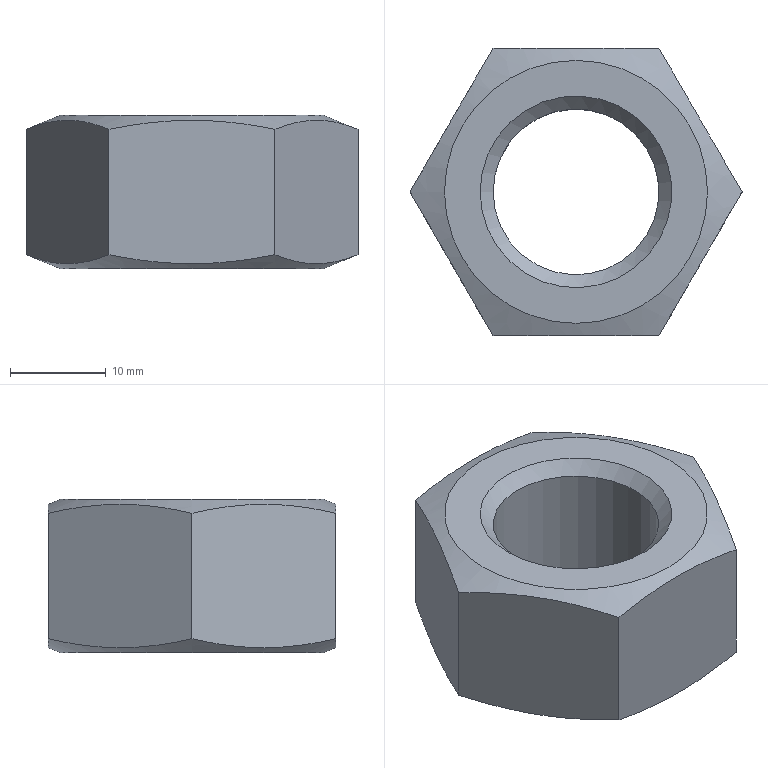Part | STEP file | 1_28 | 1 solid | 13 faces | box 34.641 x 30 x 16 mm | volume 8431 mm3 | plane 8 | cone 4 | cylinder 1 | commonest cylinder face diameters 17.294 x1
STEP:
#1=CARTESIAN_POINT('',(0.,0.,0.));
#2=DIRECTION('',(0.,0.,1.));
#3=DIRECTION('',(1.,0.,0.));
#4=AXIS2_PLACEMENT_3D('',#1,#2,#3);
#5=CARTESIAN_POINT('',(-8.647,0.,1.353));
#6=VERTEX_POINT('',#5);
#7=CARTESIAN_POINT('',(0.,0.,1.353));
#8=DIRECTION('',(0.,0.,-1.));
#9=DIRECTION('',(1.,0.,0.));
#10=AXIS2_PLACEMENT_3D('',#7,#8,#9);
#11=CIRCLE('',#10,8.647);
#12=CARTESIAN_POINT('',(0.,0.,0.6766));
#13=DIRECTION('',(0.,0.,-1.));
#14=DIRECTION('',(1.,0.,0.));
#15=AXIS2_PLACEMENT_3D('',#12,#13,#14);
#16=CONICAL_SURFACE('',#15,9.323,0.7854);
#17=CARTESIAN_POINT('',(0.,-0.6766));
#18=DIRECTION('',(1.,0.));
#19=VECTOR('',#18,1.);
#20=LINE('',#17,#19);
#21=(GEOMETRIC_REPRESENTATION_CONTEXT(2)PARAMETRIC_REPRESENTATION_CONTEXT()REPRESENTATION_CONTEXT('',''));
#22=DEFINITIONAL_REPRESENTATION('',(#20),#21);
#23=PCURVE('',#16,#22);
#24=CARTESIAN_POINT('',(0.,0.,8.));
#25=DIRECTION('',(0.,0.,-1.));
#26=DIRECTION('',(1.,0.,0.));
#27=AXIS2_PLACEMENT_3D('',#24,#25,#26);
#28=CYLINDRICAL_SURFACE('',#27,8.647);
#29=CARTESIAN_POINT('',(0.,6.647));
#30=DIRECTION('',(1.,0.));
#31=VECTOR('',#30,1.);
#32=LINE('',#29,#31);
#33=(GEOMETRIC_REPRESENTATION_CONTEXT(2)PARAMETRIC_REPRESENTATION_CONTEXT()REPRESENTATION_CONTEXT('',''));
#34=DEFINITIONAL_REPRESENTATION('',(#32),#33);
#35=PCURVE('',#28,#34);
#36=SURFACE_CURVE('',#11,(#23,#35),.PCURVE_S1.);
#37=EDGE_CURVE('',#6,#6,#36,.T.);
#38=ORIENTED_EDGE('',*,*,#37,.T.);
#39=CARTESIAN_POINT('',(-10.,0.,0.));
#40=VERTEX_POINT('',#39);
#41=CARTESIAN_POINT('',(-8.647,0.,1.353));
#42=CARTESIAN_POINT('',(-10.,0.,-0.000000001));
#43=B_SPLINE_CURVE_WITH_KNOTS('',1,(#41,#42),.UNSPECIFIED.,.F.,.F.,(2,2),(-0.9568,0.9568),.PIECEWISE_BEZIER_KNOTS.);
#44=CARTESIAN_POINT('',(9.425,0.));
#45=DIRECTION('',(0.,1.));
#46=VECTOR('',#45,1.);
#47=LINE('',#44,#46);
#48=(GEOMETRIC_REPRESENTATION_CONTEXT(2)PARAMETRIC_REPRESENTATION_CONTEXT()REPRESENTATION_CONTEXT('',''));
#49=DEFINITIONAL_REPRESENTATION('',(#47),#48);
#50=PCURVE('',#16,#49);
#51=CARTESIAN_POINT('',(3.142,0.));
#52=DIRECTION('',(0.,1.));
#53=VECTOR('',#52,1.);
#54=LINE('',#51,#53);
#55=(GEOMETRIC_REPRESENTATION_CONTEXT(2)PARAMETRIC_REPRESENTATION_CONTEXT()REPRESENTATION_CONTEXT('',''));
#56=DEFINITIONAL_REPRESENTATION('',(#54),#55);
#57=PCURVE('',#16,#56);
#58=SEAM_CURVE('',#43,(#50,#57),.PCURVE_S1.);
#59=EDGE_CURVE('',#6,#40,#58,.T.);
#60=ORIENTED_EDGE('',*,*,#59,.T.);
#61=CARTESIAN_POINT('',(0.,0.,0.));
#62=DIRECTION('',(0.,0.,-1.));
#63=DIRECTION('',(1.,0.,0.));
#64=AXIS2_PLACEMENT_3D('',#61,#62,#63);
#65=CIRCLE('',#64,10.);
#66=CARTESIAN_POINT('',(0.,0.6766));
#67=DIRECTION('',(1.,0.));
#68=VECTOR('',#67,1.);
#69=LINE('',#66,#68);
#70=(GEOMETRIC_REPRESENTATION_CONTEXT(2)PARAMETRIC_REPRESENTATION_CONTEXT()REPRESENTATION_CONTEXT('',''));
#71=DEFINITIONAL_REPRESENTATION('',(#69),#70);
#72=PCURVE('',#16,#71);
#73=CARTESIAN_POINT('',(0.,0.,0.));
#74=DIRECTION('',(0.,0.,1.));
#75=DIRECTION('',(1.,0.,0.));
#76=AXIS2_PLACEMENT_3D('',#73,#74,#75);
#77=PLANE('',#76);
#78=CARTESIAN_POINT('',(10.,0.));
#79=CARTESIAN_POINT('',(10.,-17.321));
#80=CARTESIAN_POINT('',(-5.,-8.66));
#81=CARTESIAN_POINT('',(-20.,0.));
#82=CARTESIAN_POINT('',(-5.,8.66));
#83=CARTESIAN_POINT('',(10.,17.321));
#84=CARTESIAN_POINT('',(10.,0.));
#85=(BOUNDED_CURVE()B_SPLINE_CURVE(2,(#78,#79,#80,#81,#82,#83,#84),.UNSPECIFIED.,.T.,.F.)B_SPLINE_CURVE_WITH_KNOTS((1,2,2,2,2,1),(-2.094,0.,2.094,4.189,6.283,8.378),.UNSPECIFIED.)CURVE()GEOMETRIC_REPRESENTATION_ITEM()RATIONAL_B_SPLINE_CURVE((1.,0.5,1.,0.5,1.,0.5,1.))REPRESENTATION_ITEM(''));
#86=(GEOMETRIC_REPRESENTATION_CONTEXT(2)PARAMETRIC_REPRESENTATION_CONTEXT()REPRESENTATION_CONTEXT('',''));
#87=DEFINITIONAL_REPRESENTATION('',(#85),#86);
#88=PCURVE('',#77,#87);
#89=SURFACE_CURVE('',#65,(#72,#88),.PCURVE_S1.);
#90=EDGE_CURVE('',#40,#40,#89,.T.);
#91=ORIENTED_EDGE('',*,*,#90,.F.);
#92=ORIENTED_EDGE('',*,*,#59,.F.);
#93=EDGE_LOOP('',(#38,#60,#91,#92));
#94=FACE_BOUND('',#93,.F.);
#95=ADVANCED_FACE('',(#94),#16,.F.);
#96=CARTESIAN_POINT('',(-13.72,0.,0.));
#97=VERTEX_POINT('',#96);
#98=CARTESIAN_POINT('',(0.,0.,0.));
#99=DIRECTION('',(0.,0.,1.));
#100=DIRECTION('',(1.,0.,0.));
#101=AXIS2_PLACEMENT_3D('',#98,#99,#100);
#102=CIRCLE('',#101,13.72);
#103=CARTESIAN_POINT('',(0.,0.));
#104=DIRECTION('',(1.,0.));
#105=AXIS2_PLACEMENT_2D('',#103,#104);
#106=CIRCLE('',#105,13.72);
#107=(GEOMETRIC_REPRESENTATION_CONTEXT(2)PARAMETRIC_REPRESENTATION_CONTEXT()REPRESENTATION_CONTEXT('',''));
#108=DEFINITIONAL_REPRESENTATION('',(#106),#107);
#109=PCURVE('',#77,#108);
#110=CARTESIAN_POINT('',(0.,0.,0.7273));
#111=DIRECTION('',(0.,0.,1.));
#112=DIRECTION('',(1.,0.,0.));
#113=AXIS2_PLACEMENT_3D('',#110,#111,#112);
#114=CONICAL_SURFACE('',#113,15.52,1.187);
#115=CARTESIAN_POINT('',(0.,-0.7273));
#116=DIRECTION('',(1.,0.));
#117=VECTOR('',#116,1.);
#118=LINE('',#115,#117);
#119=(GEOMETRIC_REPRESENTATION_CONTEXT(2)PARAMETRIC_REPRESENTATION_CONTEXT()REPRESENTATION_CONTEXT('',''));
#120=DEFINITIONAL_REPRESENTATION('',(#118),#119);
#121=PCURVE('',#114,#120);
#122=SURFACE_CURVE('',#102,(#109,#121),.PCURVE_S1.);
#123=EDGE_CURVE('',#97,#97,#122,.T.);
#124=ORIENTED_EDGE('',*,*,#123,.F.);
#125=EDGE_LOOP('',(#124));
#126=FACE_BOUND('',#125,.T.);
#127=ORIENTED_EDGE('',*,*,#90,.F.);
#128=EDGE_LOOP('',(#127));
#129=FACE_BOUND('',#128,.T.);
#130=ADVANCED_FACE('',(#126,#129),#77,.F.);
#131=CARTESIAN_POINT('',(-8.647,0.,14.647));
#132=VERTEX_POINT('',#131);
#133=CARTESIAN_POINT('',(0.,0.,14.647));
#134=DIRECTION('',(0.,0.,-1.));
#135=DIRECTION('',(1.,0.,0.));
#136=AXIS2_PLACEMENT_3D('',#133,#134,#135);
#137=CIRCLE('',#136,8.647);
#138=CARTESIAN_POINT('',(0.,-6.647));
#139=DIRECTION('',(1.,0.));
#140=VECTOR('',#139,1.);
#141=LINE('',#138,#140);
#142=(GEOMETRIC_REPRESENTATION_CONTEXT(2)PARAMETRIC_REPRESENTATION_CONTEXT()REPRESENTATION_CONTEXT('',''));
#143=DEFINITIONAL_REPRESENTATION('',(#141),#142);
#144=PCURVE('',#28,#143);
#145=CARTESIAN_POINT('',(0.,0.,15.323));
#146=DIRECTION('',(0.,0.,1.));
#147=DIRECTION('',(-1.,0.,0.));
#148=AXIS2_PLACEMENT_3D('',#145,#146,#147);
#149=CONICAL_SURFACE('',#148,9.323,0.7854);
#150=CARTESIAN_POINT('',(9.425,-0.6766));
#151=DIRECTION('',(-1.,0.));
#152=VECTOR('',#151,1.);
#153=LINE('',#150,#152);
#154=(GEOMETRIC_REPRESENTATION_CONTEXT(2)PARAMETRIC_REPRESENTATION_CONTEXT()REPRESENTATION_CONTEXT('',''));
#155=DEFINITIONAL_REPRESENTATION('',(#153),#154);
#156=PCURVE('',#149,#155);
#157=SURFACE_CURVE('',#137,(#144,#156),.PCURVE_S1.);
#158=EDGE_CURVE('',#132,#132,#157,.T.);
#159=ORIENTED_EDGE('',*,*,#158,.T.);
#160=CARTESIAN_POINT('',(-8.647,0.,14.647));
#161=CARTESIAN_POINT('',(-8.647,0.,1.353));
#162=B_SPLINE_CURVE_WITH_KNOTS('',1,(#160,#161),.UNSPECIFIED.,.F.,.F.,(2,2),(-6.647,6.647),.PIECEWISE_BEZIER_KNOTS.);
#163=CARTESIAN_POINT('',(9.425,0.));
#164=DIRECTION('',(0.,1.));
#165=VECTOR('',#164,1.);
#166=LINE('',#163,#165);
#167=(GEOMETRIC_REPRESENTATION_CONTEXT(2)PARAMETRIC_REPRESENTATION_CONTEXT()REPRESENTATION_CONTEXT('',''));
#168=DEFINITIONAL_REPRESENTATION('',(#166),#167);
#169=PCURVE('',#28,#168);
#170=CARTESIAN_POINT('',(3.142,0.));
#171=DIRECTION('',(0.,1.));
#172=VECTOR('',#171,1.);
#173=LINE('',#170,#172);
#174=(GEOMETRIC_REPRESENTATION_CONTEXT(2)PARAMETRIC_REPRESENTATION_CONTEXT()REPRESENTATION_CONTEXT('',''));
#175=DEFINITIONAL_REPRESENTATION('',(#173),#174);
#176=PCURVE('',#28,#175);
#177=SEAM_CURVE('',#162,(#169,#176),.PCURVE_S1.);
#178=EDGE_CURVE('',#132,#6,#177,.T.);
#179=ORIENTED_EDGE('',*,*,#178,.T.);
#180=ORIENTED_EDGE('',*,*,#37,.F.);
#181=ORIENTED_EDGE('',*,*,#178,.F.);
#182=EDGE_LOOP('',(#159,#179,#180,#181));
#183=FACE_BOUND('',#182,.F.);
#184=ADVANCED_FACE('',(#183),#28,.F.);
#185=CARTESIAN_POINT('',(-17.32,0.,1.455));
#186=VERTEX_POINT('',#185);
#187=CARTESIAN_POINT('',(-8.66,15.,1.455));
#188=VERTEX_POINT('',#187);
#189=CARTESIAN_POINT('',(-39.287,-38.047,16.553));
#190=CARTESIAN_POINT('',(-12.99,7.5,-3.881));
#191=CARTESIAN_POINT('',(13.306,53.047,16.553));
#192=(BOUNDED_CURVE()B_SPLINE_CURVE(2,(#189,#190,#191),.UNSPECIFIED.,.F.,.F.)B_SPLINE_CURVE_WITH_KNOTS((3,3),(0.,10.997),.PIECEWISE_BEZIER_KNOTS.)CURVE()GEOMETRIC_REPRESENTATION_ITEM()RATIONAL_B_SPLINE_CURVE((1.,3.646,1.))REPRESENTATION_ITEM(''));
#193=CARTESIAN_POINT('',(9.425,0.7273));
#194=CARTESIAN_POINT('',(9.41,0.6661));
#195=CARTESIAN_POINT('',(9.379,0.5509));
#196=CARTESIAN_POINT('',(9.333,0.3985));
#197=CARTESIAN_POINT('',(9.286,0.2652));
#198=CARTESIAN_POINT('',(9.239,0.1498));
#199=CARTESIAN_POINT('',(9.191,0.05157));
#200=CARTESIAN_POINT('',(9.144,-0.03038));
#201=CARTESIAN_POINT('',(9.095,-0.09663));
#202=CARTESIAN_POINT('',(9.047,-0.1477));
#203=CARTESIAN_POINT('',(8.999,-0.1839));
#204=CARTESIAN_POINT('',(8.95,-0.2055));
#205=CARTESIAN_POINT('',(8.901,-0.2127));
#206=CARTESIAN_POINT('',(8.852,-0.2055));
#207=CARTESIAN_POINT('',(8.804,-0.1839));
#208=CARTESIAN_POINT('',(8.755,-0.1477));
#209=CARTESIAN_POINT('',(8.707,-0.09663));
#210=CARTESIAN_POINT('',(8.659,-0.03038));
#211=CARTESIAN_POINT('',(8.611,0.05157));
#212=CARTESIAN_POINT('',(8.563,0.1498));
#213=CARTESIAN_POINT('',(8.516,0.2652));
#214=CARTESIAN_POINT('',(8.469,0.3985));
#215=CARTESIAN_POINT('',(8.423,0.5509));
#216=CARTESIAN_POINT('',(8.393,0.6661));
#217=CARTESIAN_POINT('',(8.378,0.7273));
#218=B_SPLINE_CURVE_WITH_KNOTS('',3,(#193,#194,#195,#196,#197,#198,#199,#200,#201,#202,#203,#204,#205,#206,#207,#208,#209,#210,#211,#212,#213,#214,#215,#216,#217),.UNSPECIFIED.,.F.,.F.,(4,1,1,1,1,1,1,1,1,1,1,1,1,1,1,1,1,1,1,1,1,1,4),(3.546,3.724,3.901,4.079,4.256,4.434,4.611,4.788,4.966,5.143,5.321,5.498,5.676,5.853,6.031,6.208,6.386,6.563,6.741,6.918,7.096,7.273,7.451),.QUASI_UNIFORM_KNOTS.);
#219=(GEOMETRIC_REPRESENTATION_CONTEXT(2)PARAMETRIC_REPRESENTATION_CONTEXT()REPRESENTATION_CONTEXT('',''));
#220=DEFINITIONAL_REPRESENTATION('',(#218),#219);
#221=PCURVE('',#114,#220);
#222=CARTESIAN_POINT('',(-17.32,0.,0.));
#223=DIRECTION('',(-0.866,0.5,0.));
#224=DIRECTION('',(0.,0.,1.));
#225=AXIS2_PLACEMENT_3D('',#222,#223,#224);
#226=PLANE('',#225);
#227=CARTESIAN_POINT('',(16.553,-43.933));
#228=CARTESIAN_POINT('',(-3.881,8.66));
#229=CARTESIAN_POINT('',(16.553,61.253));
#230=(BOUNDED_CURVE()B_SPLINE_CURVE(2,(#227,#228,#229),.UNSPECIFIED.,.F.,.F.)B_SPLINE_CURVE_WITH_KNOTS((3,3),(0.,10.997),.PIECEWISE_BEZIER_KNOTS.)CURVE()GEOMETRIC_REPRESENTATION_ITEM()RATIONAL_B_SPLINE_CURVE((1.,3.646,1.))REPRESENTATION_ITEM(''));
#231=(GEOMETRIC_REPRESENTATION_CONTEXT(2)PARAMETRIC_REPRESENTATION_CONTEXT()REPRESENTATION_CONTEXT('',''));
#232=DEFINITIONAL_REPRESENTATION('',(#230),#231);
#233=PCURVE('',#226,#232);
#234=SURFACE_CURVE('',#192,(#221,#233),.PCURVE_S1.);
#235=EDGE_CURVE('',#186,#188,#234,.T.);
#236=ORIENTED_EDGE('',*,*,#235,.T.);
#237=CARTESIAN_POINT('',(8.66,15.,1.455));
#238=VERTEX_POINT('',#237);
#239=CARTESIAN_POINT('',(-52.593,15.,16.553));
#240=CARTESIAN_POINT('',(0.,15.,-3.881));
#241=CARTESIAN_POINT('',(52.593,15.,16.553));
#242=(BOUNDED_CURVE()B_SPLINE_CURVE(2,(#239,#240,#241),.UNSPECIFIED.,.F.,.F.)B_SPLINE_CURVE_WITH_KNOTS((3,3),(0.,10.997),.PIECEWISE_BEZIER_KNOTS.)CURVE()GEOMETRIC_REPRESENTATION_ITEM()RATIONAL_B_SPLINE_CURVE((1.,3.646,1.))REPRESENTATION_ITEM(''));
#243=CARTESIAN_POINT('',(8.378,0.7273));
#244=CARTESIAN_POINT('',(8.362,0.6661));
#245=CARTESIAN_POINT('',(8.332,0.5509));
#246=CARTESIAN_POINT('',(8.286,0.3985));
#247=CARTESIAN_POINT('',(8.239,0.2652));
#248=CARTESIAN_POINT('',(8.192,0.1498));
#249=CARTESIAN_POINT('',(8.144,0.05157));
#250=CARTESIAN_POINT('',(8.096,-0.03038));
#251=CARTESIAN_POINT('',(8.048,-0.09663));
#252=CARTESIAN_POINT('',(8.,-0.1477));
#253=CARTESIAN_POINT('',(7.951,-0.1839));
#254=CARTESIAN_POINT('',(7.903,-0.2055));
#255=CARTESIAN_POINT('',(7.854,-0.2127));
#256=CARTESIAN_POINT('',(7.805,-0.2055));
#257=CARTESIAN_POINT('',(7.757,-0.1839));
#258=CARTESIAN_POINT('',(7.708,-0.1477));
#259=CARTESIAN_POINT('',(7.66,-0.09663));
#260=CARTESIAN_POINT('',(7.612,-0.03038));
#261=CARTESIAN_POINT('',(7.564,0.05157));
#262=CARTESIAN_POINT('',(7.516,0.1498));
#263=CARTESIAN_POINT('',(7.469,0.2652));
#264=CARTESIAN_POINT('',(7.422,0.3985));
#265=CARTESIAN_POINT('',(7.376,0.5509));
#266=CARTESIAN_POINT('',(7.346,0.6661));
#267=CARTESIAN_POINT('',(7.33,0.7273));
#268=B_SPLINE_CURVE_WITH_KNOTS('',3,(#243,#244,#245,#246,#247,#248,#249,#250,#251,#252,#253,#254,#255,#256,#257,#258,#259,#260,#261,#262,#263,#264,#265,#266,#267),.UNSPECIFIED.,.F.,.F.,(4,1,1,1,1,1,1,1,1,1,1,1,1,1,1,1,1,1,1,1,1,1,4),(3.546,3.724,3.901,4.079,4.256,4.434,4.611,4.788,4.966,5.143,5.321,5.498,5.676,5.853,6.031,6.208,6.386,6.563,6.741,6.918,7.096,7.273,7.451),.QUASI_UNIFORM_KNOTS.);
#269=(GEOMETRIC_REPRESENTATION_CONTEXT(2)PARAMETRIC_REPRESENTATION_CONTEXT()REPRESENTATION_CONTEXT('',''));
#270=DEFINITIONAL_REPRESENTATION('',(#268),#269);
#271=PCURVE('',#114,#270);
#272=CARTESIAN_POINT('',(-8.66,15.,0.));
#273=DIRECTION('',(0.,1.,0.));
#274=DIRECTION('',(0.,0.,1.));
#275=AXIS2_PLACEMENT_3D('',#272,#273,#274);
#276=PLANE('',#275);
#277=CARTESIAN_POINT('',(16.553,-43.933));
#278=CARTESIAN_POINT('',(-3.881,8.66));
#279=CARTESIAN_POINT('',(16.553,61.253));
#280=(BOUNDED_CURVE()B_SPLINE_CURVE(2,(#277,#278,#279),.UNSPECIFIED.,.F.,.F.)B_SPLINE_CURVE_WITH_KNOTS((3,3),(0.,10.997),.PIECEWISE_BEZIER_KNOTS.)CURVE()GEOMETRIC_REPRESENTATION_ITEM()RATIONAL_B_SPLINE_CURVE((1.,3.646,1.))REPRESENTATION_ITEM(''));
#281=(GEOMETRIC_REPRESENTATION_CONTEXT(2)PARAMETRIC_REPRESENTATION_CONTEXT()REPRESENTATION_CONTEXT('',''));
#282=DEFINITIONAL_REPRESENTATION('',(#280),#281);
#283=PCURVE('',#276,#282);
#284=SURFACE_CURVE('',#242,(#271,#283),.PCURVE_S1.);
#285=EDGE_CURVE('',#188,#238,#284,.T.);
#286=ORIENTED_EDGE('',*,*,#285,.T.);
#287=CARTESIAN_POINT('',(17.32,0.,1.455));
#288=VERTEX_POINT('',#287);
#289=CARTESIAN_POINT('',(-13.306,53.047,16.553));
#290=CARTESIAN_POINT('',(12.99,7.5,-3.881));
#291=CARTESIAN_POINT('',(39.287,-38.047,16.553));
#292=(BOUNDED_CURVE()B_SPLINE_CURVE(2,(#289,#290,#291),.UNSPECIFIED.,.F.,.F.)B_SPLINE_CURVE_WITH_KNOTS((3,3),(0.,10.997),.PIECEWISE_BEZIER_KNOTS.)CURVE()GEOMETRIC_REPRESENTATION_ITEM()RATIONAL_B_SPLINE_CURVE((1.,3.646,1.))REPRESENTATION_ITEM(''));
#293=CARTESIAN_POINT('',(7.33,0.7273));
#294=CARTESIAN_POINT('',(7.315,0.6661));
#295=CARTESIAN_POINT('',(7.285,0.5509));
#296=CARTESIAN_POINT('',(7.238,0.3985));
#297=CARTESIAN_POINT('',(7.192,0.2652));
#298=CARTESIAN_POINT('',(7.145,0.1498));
#299=CARTESIAN_POINT('',(7.097,0.05157));
#300=CARTESIAN_POINT('',(7.049,-0.03038));
#301=CARTESIAN_POINT('',(7.001,-0.09663));
#302=CARTESIAN_POINT('',(6.953,-0.1477));
#303=CARTESIAN_POINT('',(6.904,-0.1839));
#304=CARTESIAN_POINT('',(6.856,-0.2055));
#305=CARTESIAN_POINT('',(6.807,-0.2127));
#306=CARTESIAN_POINT('',(6.758,-0.2055));
#307=CARTESIAN_POINT('',(6.709,-0.1839));
#308=CARTESIAN_POINT('',(6.661,-0.1477));
#309=CARTESIAN_POINT('',(6.612,-0.09663));
#310=CARTESIAN_POINT('',(6.564,-0.03038));
#311=CARTESIAN_POINT('',(6.516,0.05157));
#312=CARTESIAN_POINT('',(6.469,0.1498));
#313=CARTESIAN_POINT('',(6.422,0.2652));
#314=CARTESIAN_POINT('',(6.375,0.3985));
#315=CARTESIAN_POINT('',(6.329,0.5509));
#316=CARTESIAN_POINT('',(6.298,0.6661));
#317=CARTESIAN_POINT('',(6.283,0.7273));
#318=B_SPLINE_CURVE_WITH_KNOTS('',3,(#293,#294,#295,#296,#297,#298,#299,#300,#301,#302,#303,#304,#305,#306,#307,#308,#309,#310,#311,#312,#313,#314,#315,#316,#317),.UNSPECIFIED.,.F.,.F.,(4,1,1,1,1,1,1,1,1,1,1,1,1,1,1,1,1,1,1,1,1,1,4),(3.546,3.724,3.901,4.079,4.256,4.434,4.611,4.788,4.966,5.143,5.321,5.498,5.676,5.853,6.031,6.208,6.386,6.563,6.741,6.918,7.096,7.273,7.451),.QUASI_UNIFORM_KNOTS.);
#319=(GEOMETRIC_REPRESENTATION_CONTEXT(2)PARAMETRIC_REPRESENTATION_CONTEXT()REPRESENTATION_CONTEXT('',''));
#320=DEFINITIONAL_REPRESENTATION('',(#318),#319);
#321=PCURVE('',#114,#320);
#322=CARTESIAN_POINT('',(8.66,15.,0.));
#323=DIRECTION('',(0.866,0.5,0.));
#324=DIRECTION('',(0.,0.,-1.));
#325=AXIS2_PLACEMENT_3D('',#322,#323,#324);
#326=PLANE('',#325);
#327=CARTESIAN_POINT('',(-16.553,43.933));
#328=CARTESIAN_POINT('',(3.881,-8.66));
#329=CARTESIAN_POINT('',(-16.553,-61.253));
#330=(BOUNDED_CURVE()B_SPLINE_CURVE(2,(#327,#328,#329),.UNSPECIFIED.,.F.,.F.)B_SPLINE_CURVE_WITH_KNOTS((3,3),(0.,10.997),.PIECEWISE_BEZIER_KNOTS.)CURVE()GEOMETRIC_REPRESENTATION_ITEM()RATIONAL_B_SPLINE_CURVE((1.,3.646,1.))REPRESENTATION_ITEM(''));
#331=(GEOMETRIC_REPRESENTATION_CONTEXT(2)PARAMETRIC_REPRESENTATION_CONTEXT()REPRESENTATION_CONTEXT('',''));
#332=DEFINITIONAL_REPRESENTATION('',(#330),#331);
#333=PCURVE('',#326,#332);
#334=SURFACE_CURVE('',#292,(#321,#333),.PCURVE_S1.);
#335=EDGE_CURVE('',#238,#288,#334,.T.);
#336=ORIENTED_EDGE('',*,*,#335,.T.);
#337=CARTESIAN_POINT('',(8.66,-15.,1.455));
#338=VERTEX_POINT('',#337);
#339=CARTESIAN_POINT('',(39.287,38.047,16.553));
#340=CARTESIAN_POINT('',(12.99,-7.5,-3.881));
#341=CARTESIAN_POINT('',(-13.306,-53.047,16.553));
#342=(BOUNDED_CURVE()B_SPLINE_CURVE(2,(#339,#340,#341),.UNSPECIFIED.,.F.,.F.)B_SPLINE_CURVE_WITH_KNOTS((3,3),(0.,10.997),.PIECEWISE_BEZIER_KNOTS.)CURVE()GEOMETRIC_REPRESENTATION_ITEM()RATIONAL_B_SPLINE_CURVE((1.,3.646,1.))REPRESENTATION_ITEM(''));
#343=CARTESIAN_POINT('',(6.283,0.7273));
#344=CARTESIAN_POINT('',(6.268,0.6661));
#345=CARTESIAN_POINT('',(6.238,0.5509));
#346=CARTESIAN_POINT('',(6.191,0.3985));
#347=CARTESIAN_POINT('',(6.145,0.2652));
#348=CARTESIAN_POINT('',(6.097,0.1498));
#349=CARTESIAN_POINT('',(6.05,0.05157));
#350=CARTESIAN_POINT('',(6.002,-0.03038));
#351=CARTESIAN_POINT('',(5.954,-0.09663));
#352=CARTESIAN_POINT('',(5.906,-0.1477));
#353=CARTESIAN_POINT('',(5.857,-0.1839));
#354=CARTESIAN_POINT('',(5.808,-0.2055));
#355=CARTESIAN_POINT('',(5.76,-0.2127));
#356=CARTESIAN_POINT('',(5.711,-0.2055));
#357=CARTESIAN_POINT('',(5.662,-0.1839));
#358=CARTESIAN_POINT('',(5.614,-0.1477));
#359=CARTESIAN_POINT('',(5.565,-0.09663));
#360=CARTESIAN_POINT('',(5.517,-0.03038));
#361=CARTESIAN_POINT('',(5.469,0.05157));
#362=CARTESIAN_POINT('',(5.422,0.1498));
#363=CARTESIAN_POINT('',(5.375,0.2652));
#364=CARTESIAN_POINT('',(5.328,0.3985));
#365=CARTESIAN_POINT('',(5.282,0.5509));
#366=CARTESIAN_POINT('',(5.251,0.6661));
#367=CARTESIAN_POINT('',(5.236,0.7273));
#368=B_SPLINE_CURVE_WITH_KNOTS('',3,(#343,#344,#345,#346,#347,#348,#349,#350,#351,#352,#353,#354,#355,#356,#357,#358,#359,#360,#361,#362,#363,#364,#365,#366,#367),.UNSPECIFIED.,.F.,.F.,(4,1,1,1,1,1,1,1,1,1,1,1,1,1,1,1,1,1,1,1,1,1,4),(3.546,3.724,3.901,4.079,4.256,4.434,4.611,4.788,4.966,5.143,5.321,5.498,5.676,5.853,6.031,6.208,6.386,6.563,6.741,6.918,7.096,7.273,7.451),.QUASI_UNIFORM_KNOTS.);
#369=(GEOMETRIC_REPRESENTATION_CONTEXT(2)PARAMETRIC_REPRESENTATION_CONTEXT()REPRESENTATION_CONTEXT('',''));
#370=DEFINITIONAL_REPRESENTATION('',(#368),#369);
#371=PCURVE('',#114,#370);
#372=CARTESIAN_POINT('',(17.32,0.,0.));
#373=DIRECTION('',(0.866,-0.5,0.));
#374=DIRECTION('',(0.,0.,-1.));
#375=AXIS2_PLACEMENT_3D('',#372,#373,#374);
#376=PLANE('',#375);
#377=CARTESIAN_POINT('',(-16.553,43.933));
#378=CARTESIAN_POINT('',(3.881,-8.66));
#379=CARTESIAN_POINT('',(-16.553,-61.253));
#380=(BOUNDED_CURVE()B_SPLINE_CURVE(2,(#377,#378,#379),.UNSPECIFIED.,.F.,.F.)B_SPLINE_CURVE_WITH_KNOTS((3,3),(0.,10.997),.PIECEWISE_BEZIER_KNOTS.)CURVE()GEOMETRIC_REPRESENTATION_ITEM()RATIONAL_B_SPLINE_CURVE((1.,3.646,1.))REPRESENTATION_ITEM(''));
#381=(GEOMETRIC_REPRESENTATION_CONTEXT(2)PARAMETRIC_REPRESENTATION_CONTEXT()REPRESENTATION_CONTEXT('',''));
#382=DEFINITIONAL_REPRESENTATION('',(#380),#381);
#383=PCURVE('',#376,#382);
#384=SURFACE_CURVE('',#342,(#371,#383),.PCURVE_S1.);
#385=EDGE_CURVE('',#288,#338,#384,.T.);
#386=ORIENTED_EDGE('',*,*,#385,.T.);
#387=CARTESIAN_POINT('',(-8.66,-15.,1.455));
#388=VERTEX_POINT('',#387);
#389=CARTESIAN_POINT('',(52.593,-15.,16.553));
#390=CARTESIAN_POINT('',(0.,-15.,-3.881));
#391=CARTESIAN_POINT('',(-52.593,-15.,16.553));
#392=(BOUNDED_CURVE()B_SPLINE_CURVE(2,(#389,#390,#391),.UNSPECIFIED.,.F.,.F.)B_SPLINE_CURVE_WITH_KNOTS((3,3),(0.,10.997),.PIECEWISE_BEZIER_KNOTS.)CURVE()GEOMETRIC_REPRESENTATION_ITEM()RATIONAL_B_SPLINE_CURVE((1.,3.646,1.))REPRESENTATION_ITEM(''));
#393=CARTESIAN_POINT('',(5.236,0.7273));
#394=CARTESIAN_POINT('',(5.221,0.6661));
#395=CARTESIAN_POINT('',(5.19,0.5509));
#396=CARTESIAN_POINT('',(5.144,0.3985));
#397=CARTESIAN_POINT('',(5.097,0.2652));
#398=CARTESIAN_POINT('',(5.05,0.1498));
#399=CARTESIAN_POINT('',(5.003,0.05157));
#400=CARTESIAN_POINT('',(4.955,-0.03038));
#401=CARTESIAN_POINT('',(4.907,-0.09663));
#402=CARTESIAN_POINT('',(4.858,-0.1477));
#403=CARTESIAN_POINT('',(4.81,-0.1839));
#404=CARTESIAN_POINT('',(4.761,-0.2055));
#405=CARTESIAN_POINT('',(4.712,-0.2127));
#406=CARTESIAN_POINT('',(4.664,-0.2055));
#407=CARTESIAN_POINT('',(4.615,-0.1839));
#408=CARTESIAN_POINT('',(4.566,-0.1477));
#409=CARTESIAN_POINT('',(4.518,-0.09663));
#410=CARTESIAN_POINT('',(4.47,-0.03038));
#411=CARTESIAN_POINT('',(4.422,0.05157));
#412=CARTESIAN_POINT('',(4.375,0.1498));
#413=CARTESIAN_POINT('',(4.327,0.2652));
#414=CARTESIAN_POINT('',(4.281,0.3985));
#415=CARTESIAN_POINT('',(4.234,0.5509));
#416=CARTESIAN_POINT('',(4.204,0.6661));
#417=CARTESIAN_POINT('',(4.189,0.7273));
#418=B_SPLINE_CURVE_WITH_KNOTS('',3,(#393,#394,#395,#396,#397,#398,#399,#400,#401,#402,#403,#404,#405,#406,#407,#408,#409,#410,#411,#412,#413,#414,#415,#416,#417),.UNSPECIFIED.,.F.,.F.,(4,1,1,1,1,1,1,1,1,1,1,1,1,1,1,1,1,1,1,1,1,1,4),(3.546,3.724,3.901,4.079,4.256,4.434,4.611,4.788,4.966,5.143,5.321,5.498,5.676,5.853,6.031,6.208,6.386,6.563,6.741,6.918,7.096,7.273,7.451),.QUASI_UNIFORM_KNOTS.);
#419=(GEOMETRIC_REPRESENTATION_CONTEXT(2)PARAMETRIC_REPRESENTATION_CONTEXT()REPRESENTATION_CONTEXT('',''));
#420=DEFINITIONAL_REPRESENTATION('',(#418),#419);
#421=PCURVE('',#114,#420);
#422=CARTESIAN_POINT('',(8.66,-15.,0.));
#423=DIRECTION('',(0.,-1.,0.));
#424=DIRECTION('',(0.,0.,-1.));
#425=AXIS2_PLACEMENT_3D('',#422,#423,#424);
#426=PLANE('',#425);
#427=CARTESIAN_POINT('',(-16.553,43.933));
#428=CARTESIAN_POINT('',(3.881,-8.66));
#429=CARTESIAN_POINT('',(-16.553,-61.253));
#430=(BOUNDED_CURVE()B_SPLINE_CURVE(2,(#427,#428,#429),.UNSPECIFIED.,.F.,.F.)B_SPLINE_CURVE_WITH_KNOTS((3,3),(0.,10.997),.PIECEWISE_BEZIER_KNOTS.)CURVE()GEOMETRIC_REPRESENTATION_ITEM()RATIONAL_B_SPLINE_CURVE((1.,3.646,1.))REPRESENTATION_ITEM(''));
#431=(GEOMETRIC_REPRESENTATION_CONTEXT(2)PARAMETRIC_REPRESENTATION_CONTEXT()REPRESENTATION_CONTEXT('',''));
#432=DEFINITIONAL_REPRESENTATION('',(#430),#431);
#433=PCURVE('',#426,#432);
#434=SURFACE_CURVE('',#392,(#421,#433),.PCURVE_S1.);
#435=EDGE_CURVE('',#338,#388,#434,.T.);
#436=ORIENTED_EDGE('',*,*,#435,.T.);
#437=CARTESIAN_POINT('',(13.306,-53.047,16.553));
#438=CARTESIAN_POINT('',(-12.99,-7.5,-3.881));
#439=CARTESIAN_POINT('',(-39.287,38.047,16.553));
#440=(BOUNDED_CURVE()B_SPLINE_CURVE(2,(#437,#438,#439),.UNSPECIFIED.,.F.,.F.)B_SPLINE_CURVE_WITH_KNOTS((3,3),(0.,10.997),.PIECEWISE_BEZIER_KNOTS.)CURVE()GEOMETRIC_REPRESENTATION_ITEM()RATIONAL_B_SPLINE_CURVE((1.,3.646,1.))REPRESENTATION_ITEM(''));
#441=CARTESIAN_POINT('',(4.189,0.7273));
#442=CARTESIAN_POINT('',(4.174,0.6661));
#443=CARTESIAN_POINT('',(4.143,0.5509));
#444=CARTESIAN_POINT('',(4.097,0.3985));
#445=CARTESIAN_POINT('',(4.05,0.2652));
#446=CARTESIAN_POINT('',(4.003,0.1498));
#447=CARTESIAN_POINT('',(3.956,0.05157));
#448=CARTESIAN_POINT('',(3.908,-0.03038));
#449=CARTESIAN_POINT('',(3.859,-0.09663));
#450=CARTESIAN_POINT('',(3.811,-0.1477));
#451=CARTESIAN_POINT('',(3.763,-0.1839));
#452=CARTESIAN_POINT('',(3.714,-0.2055));
#453=CARTESIAN_POINT('',(3.665,-0.2127));
#454=CARTESIAN_POINT('',(3.616,-0.2055));
#455=CARTESIAN_POINT('',(3.568,-0.1839));
#456=CARTESIAN_POINT('',(3.519,-0.1477));
#457=CARTESIAN_POINT('',(3.471,-0.09663));
#458=CARTESIAN_POINT('',(3.423,-0.03038));
#459=CARTESIAN_POINT('',(3.375,0.05157));
#460=CARTESIAN_POINT('',(3.327,0.1498));
#461=CARTESIAN_POINT('',(3.28,0.2652));
#462=CARTESIAN_POINT('',(3.233,0.3985));
#463=CARTESIAN_POINT('',(3.187,0.5509));
#464=CARTESIAN_POINT('',(3.157,0.6661));
#465=CARTESIAN_POINT('',(3.142,0.7273));
#466=B_SPLINE_CURVE_WITH_KNOTS('',3,(#441,#442,#443,#444,#445,#446,#447,#448,#449,#450,#451,#452,#453,#454,#455,#456,#457,#458,#459,#460,#461,#462,#463,#464,#465),.UNSPECIFIED.,.F.,.F.,(4,1,1,1,1,1,1,1,1,1,1,1,1,1,1,1,1,1,1,1,1,1,4),(3.546,3.724,3.901,4.079,4.256,4.434,4.611,4.788,4.966,5.143,5.321,5.498,5.676,5.853,6.031,6.208,6.386,6.563,6.741,6.918,7.096,7.273,7.451),.QUASI_UNIFORM_KNOTS.);
#467=(GEOMETRIC_REPRESENTATION_CONTEXT(2)PARAMETRIC_REPRESENTATION_CONTEXT()REPRESENTATION_CONTEXT('',''));
#468=DEFINITIONAL_REPRESENTATION('',(#466),#467);
#469=PCURVE('',#114,#468);
#470=CARTESIAN_POINT('',(-8.66,-15.,0.));
#471=DIRECTION('',(-0.866,-0.5,0.));
#472=DIRECTION('',(0.,0.,1.));
#473=AXIS2_PLACEMENT_3D('',#470,#471,#472);
#474=PLANE('',#473);
#475=CARTESIAN_POINT('',(16.553,-43.933));
#476=CARTESIAN_POINT('',(-3.881,8.66));
#477=CARTESIAN_POINT('',(16.553,61.253));
#478=(BOUNDED_CURVE()B_SPLINE_CURVE(2,(#475,#476,#477),.UNSPECIFIED.,.F.,.F.)B_SPLINE_CURVE_WITH_KNOTS((3,3),(0.,10.997),.PIECEWISE_BEZIER_KNOTS.)CURVE()GEOMETRIC_REPRESENTATION_ITEM()RATIONAL_B_SPLINE_CURVE((1.,3.646,1.))REPRESENTATION_ITEM(''));
#479=(GEOMETRIC_REPRESENTATION_CONTEXT(2)PARAMETRIC_REPRESENTATION_CONTEXT()REPRESENTATION_CONTEXT('',''));
#480=DEFINITIONAL_REPRESENTATION('',(#478),#479);
#481=PCURVE('',#474,#480);
#482=SURFACE_CURVE('',#440,(#469,#481),.PCURVE_S1.);
#483=EDGE_CURVE('',#388,#186,#482,.T.);
#484=ORIENTED_EDGE('',*,*,#483,.T.);
#485=CARTESIAN_POINT('',(-13.72,0.,-0.000000002));
#486=CARTESIAN_POINT('',(-17.32,0.,1.455));
#487=B_SPLINE_CURVE_WITH_KNOTS('',1,(#485,#486),.UNSPECIFIED.,.F.,.F.,(2,2),(-1.941,1.941),.PIECEWISE_BEZIER_KNOTS.);
#488=CARTESIAN_POINT('',(3.142,0.));
#489=DIRECTION('',(0.,1.));
#490=VECTOR('',#489,1.);
#491=LINE('',#488,#490);
#492=(GEOMETRIC_REPRESENTATION_CONTEXT(2)PARAMETRIC_REPRESENTATION_CONTEXT()REPRESENTATION_CONTEXT('',''));
#493=DEFINITIONAL_REPRESENTATION('',(#491),#492);
#494=PCURVE('',#114,#493);
#495=CARTESIAN_POINT('',(9.425,0.));
#496=DIRECTION('',(0.,1.));
#497=VECTOR('',#496,1.);
#498=LINE('',#495,#497);
#499=(GEOMETRIC_REPRESENTATION_CONTEXT(2)PARAMETRIC_REPRESENTATION_CONTEXT()REPRESENTATION_CONTEXT('',''));
#500=DEFINITIONAL_REPRESENTATION('',(#498),#499);
#501=PCURVE('',#114,#500);
#502=SEAM_CURVE('',#487,(#494,#501),.PCURVE_S1.);
#503=EDGE_CURVE('',#97,#186,#502,.T.);
#504=ORIENTED_EDGE('',*,*,#503,.F.);
#505=ORIENTED_EDGE('',*,*,#123,.T.);
#506=ORIENTED_EDGE('',*,*,#503,.T.);
#507=EDGE_LOOP('',(#236,#286,#336,#386,#436,#484,#504,#505,#506));
#508=FACE_BOUND('',#507,.T.);
#509=ADVANCED_FACE('',(#508),#114,.T.);
#510=CARTESIAN_POINT('',(-10.,0.,16.));
#511=VERTEX_POINT('',#510);
#512=CARTESIAN_POINT('',(0.,0.,16.));
#513=DIRECTION('',(0.,0.,1.));
#514=DIRECTION('',(1.,0.,0.));
#515=AXIS2_PLACEMENT_3D('',#512,#513,#514);
#516=CIRCLE('',#515,10.);
#517=CARTESIAN_POINT('',(-3.142,0.6766));
#518=DIRECTION('',(1.,0.));
#519=VECTOR('',#518,1.);
#520=LINE('',#517,#519);
#521=(GEOMETRIC_REPRESENTATION_CONTEXT(2)PARAMETRIC_REPRESENTATION_CONTEXT()REPRESENTATION_CONTEXT('',''));
#522=DEFINITIONAL_REPRESENTATION('',(#520),#521);
#523=PCURVE('',#149,#522);
#524=CARTESIAN_POINT('',(0.,0.,16.));
#525=DIRECTION('',(0.,0.,1.));
#526=DIRECTION('',(1.,0.,0.));
#527=AXIS2_PLACEMENT_3D('',#524,#525,#526);
#528=PLANE('',#527);
#529=CARTESIAN_POINT('',(0.,0.));
#530=DIRECTION('',(1.,0.));
#531=AXIS2_PLACEMENT_2D('',#529,#530);
#532=CIRCLE('',#531,10.);
#533=(GEOMETRIC_REPRESENTATION_CONTEXT(2)PARAMETRIC_REPRESENTATION_CONTEXT()REPRESENTATION_CONTEXT('',''));
#534=DEFINITIONAL_REPRESENTATION('',(#532),#533);
#535=PCURVE('',#528,#534);
#536=SURFACE_CURVE('',#516,(#523,#535),.PCURVE_S1.);
#537=EDGE_CURVE('',#511,#511,#536,.T.);
#538=ORIENTED_EDGE('',*,*,#537,.F.);
#539=CARTESIAN_POINT('',(-8.647,0.,14.647));
#540=CARTESIAN_POINT('',(-10.,0.,16.));
#541=B_SPLINE_CURVE_WITH_KNOTS('',1,(#539,#540),.UNSPECIFIED.,.F.,.F.,(2,2),(-0.9568,0.9568),.PIECEWISE_BEZIER_KNOTS.);
#542=CARTESIAN_POINT('',(0.,0.));
#543=DIRECTION('',(0.,1.));
#544=VECTOR('',#543,1.);
#545=LINE('',#542,#544);
#546=(GEOMETRIC_REPRESENTATION_CONTEXT(2)PARAMETRIC_REPRESENTATION_CONTEXT()REPRESENTATION_CONTEXT('',''));
#547=DEFINITIONAL_REPRESENTATION('',(#545),#546);
#548=PCURVE('',#149,#547);
#549=CARTESIAN_POINT('',(6.283,0.));
#550=DIRECTION('',(0.,1.));
#551=VECTOR('',#550,1.);
#552=LINE('',#549,#551);
#553=(GEOMETRIC_REPRESENTATION_CONTEXT(2)PARAMETRIC_REPRESENTATION_CONTEXT()REPRESENTATION_CONTEXT('',''));
#554=DEFINITIONAL_REPRESENTATION('',(#552),#553);
#555=PCURVE('',#149,#554);
#556=SEAM_CURVE('',#541,(#548,#555),.PCURVE_S1.);
#557=EDGE_CURVE('',#132,#511,#556,.T.);
#558=ORIENTED_EDGE('',*,*,#557,.F.);
#559=ORIENTED_EDGE('',*,*,#158,.F.);
#560=ORIENTED_EDGE('',*,*,#557,.T.);
#561=EDGE_LOOP('',(#538,#558,#559,#560));
#562=FACE_BOUND('',#561,.F.);
#563=ADVANCED_FACE('',(#562),#149,.F.);
#564=CARTESIAN_POINT('',(-8.66,15.,14.545));
#565=VERTEX_POINT('',#564);
#566=CARTESIAN_POINT('',(-17.32,0.,14.545));
#567=VERTEX_POINT('',#566);
#568=CARTESIAN_POINT('',(14.26,54.699,-1.295));
#569=CARTESIAN_POINT('',(-12.99,7.5,19.935));
#570=CARTESIAN_POINT('',(-40.241,-39.699,-1.295));
#571=(BOUNDED_CURVE()B_SPLINE_CURVE(2,(#568,#569,#570),.UNSPECIFIED.,.F.,.F.)B_SPLINE_CURVE_WITH_KNOTS((3,3),(0.,11.405),.PIECEWISE_BEZIER_KNOTS.)CURVE()GEOMETRIC_REPRESENTATION_ITEM()RATIONAL_B_SPLINE_CURVE((1.,3.768,1.))REPRESENTATION_ITEM(''));
#572=CARTESIAN_POINT('',(-1.295,63.161));
#573=CARTESIAN_POINT('',(19.935,8.66));
#574=CARTESIAN_POINT('',(-1.295,-45.84));
#575=(BOUNDED_CURVE()B_SPLINE_CURVE(2,(#572,#573,#574),.UNSPECIFIED.,.F.,.F.)B_SPLINE_CURVE_WITH_KNOTS((3,3),(0.,11.405),.PIECEWISE_BEZIER_KNOTS.)CURVE()GEOMETRIC_REPRESENTATION_ITEM()RATIONAL_B_SPLINE_CURVE((1.,3.768,1.))REPRESENTATION_ITEM(''));
#576=(GEOMETRIC_REPRESENTATION_CONTEXT(2)PARAMETRIC_REPRESENTATION_CONTEXT()REPRESENTATION_CONTEXT('',''));
#577=DEFINITIONAL_REPRESENTATION('',(#575),#576);
#578=PCURVE('',#226,#577);
#579=CARTESIAN_POINT('',(0.,0.,15.273));
#580=DIRECTION('',(0.,0.,-1.));
#581=DIRECTION('',(-1.,0.,0.));
#582=AXIS2_PLACEMENT_3D('',#579,#580,#581);
#583=CONICAL_SURFACE('',#582,15.52,1.187);
#584=CARTESIAN_POINT('',(1.047,0.7273));
#585=CARTESIAN_POINT('',(1.032,0.6661));
#586=CARTESIAN_POINT('',(1.002,0.5509));
#587=CARTESIAN_POINT('',(0.9553,0.3985));
#588=CARTESIAN_POINT('',(0.9086,0.2652));
#589=CARTESIAN_POINT('',(0.8614,0.1498));
#590=CARTESIAN_POINT('',(0.8139,0.05157));
#591=CARTESIAN_POINT('',(0.766,-0.03038));
#592=CARTESIAN_POINT('',(0.7179,-0.09663));
#593=CARTESIAN_POINT('',(0.6695,-0.1477));
#594=CARTESIAN_POINT('',(0.621,-0.1839));
#595=CARTESIAN_POINT('',(0.5723,-0.2055));
#596=CARTESIAN_POINT('',(0.5236,-0.2127));
#597=CARTESIAN_POINT('',(0.4749,-0.2055));
#598=CARTESIAN_POINT('',(0.4262,-0.1839));
#599=CARTESIAN_POINT('',(0.3777,-0.1477));
#600=CARTESIAN_POINT('',(0.3293,-0.09663));
#601=CARTESIAN_POINT('',(0.2812,-0.03038));
#602=CARTESIAN_POINT('',(0.2333,0.05157));
#603=CARTESIAN_POINT('',(0.1858,0.1498));
#604=CARTESIAN_POINT('',(0.1386,0.2652));
#605=CARTESIAN_POINT('',(0.09189,0.3985));
#606=CARTESIAN_POINT('',(0.04564,0.5509));
#607=CARTESIAN_POINT('',(0.01515,0.6661));
#608=CARTESIAN_POINT('',(0.,0.7273));
#609=B_SPLINE_CURVE_WITH_KNOTS('',3,(#584,#585,#586,#587,#588,#589,#590,#591,#592,#593,#594,#595,#596,#597,#598,#599,#600,#601,#602,#603,#604,#605,#606,#607,#608),.UNSPECIFIED.,.F.,.F.,(4,1,1,1,1,1,1,1,1,1,1,1,1,1,1,1,1,1,1,1,1,1,4),(3.697,3.879,4.062,4.244,4.426,4.609,4.791,4.973,5.156,5.338,5.52,5.702,5.885,6.067,6.249,6.432,6.614,6.796,6.979,7.161,7.343,7.525,7.708),.QUASI_UNIFORM_KNOTS.);
#610=(GEOMETRIC_REPRESENTATION_CONTEXT(2)PARAMETRIC_REPRESENTATION_CONTEXT()REPRESENTATION_CONTEXT('',''));
#611=DEFINITIONAL_REPRESENTATION('',(#609),#610);
#612=PCURVE('',#583,#611);
#613=SURFACE_CURVE('',#571,(#578,#612),.PCURVE_S1.);
#614=EDGE_CURVE('',#565,#567,#613,.T.);
#615=ORIENTED_EDGE('',*,*,#614,.F.);
#616=CARTESIAN_POINT('',(-8.66,15.,1.455));
#617=DIRECTION('',(0.,0.,1.));
#618=VECTOR('',#617,1.);
#619=LINE('',#616,#618);
#620=CARTESIAN_POINT('',(1.455,17.32));
#621=DIRECTION('',(1.,0.));
#622=VECTOR('',#621,1.);
#623=LINE('',#620,#622);
#624=(GEOMETRIC_REPRESENTATION_CONTEXT(2)PARAMETRIC_REPRESENTATION_CONTEXT()REPRESENTATION_CONTEXT('',''));
#625=DEFINITIONAL_REPRESENTATION('',(#623),#624);
#626=PCURVE('',#226,#625);
#627=CARTESIAN_POINT('',(1.455,0.));
#628=DIRECTION('',(1.,0.));
#629=VECTOR('',#628,1.);
#630=LINE('',#627,#629);
#631=(GEOMETRIC_REPRESENTATION_CONTEXT(2)PARAMETRIC_REPRESENTATION_CONTEXT()REPRESENTATION_CONTEXT('',''));
#632=DEFINITIONAL_REPRESENTATION('',(#630),#631);
#633=PCURVE('',#276,#632);
#634=SURFACE_CURVE('',#619,(#626,#633),.PCURVE_S1.);
#635=EDGE_CURVE('',#188,#565,#634,.T.);
#636=ORIENTED_EDGE('',*,*,#635,.F.);
#637=ORIENTED_EDGE('',*,*,#235,.F.);
#638=CARTESIAN_POINT('',(-17.32,0.,1.455));
#639=DIRECTION('',(0.,0.,1.));
#640=VECTOR('',#639,1.);
#641=LINE('',#638,#640);
#642=CARTESIAN_POINT('',(1.455,0.));
#643=DIRECTION('',(1.,0.));
#644=VECTOR('',#643,1.);
#645=LINE('',#642,#644);
#646=(GEOMETRIC_REPRESENTATION_CONTEXT(2)PARAMETRIC_REPRESENTATION_CONTEXT()REPRESENTATION_CONTEXT('',''));
#647=DEFINITIONAL_REPRESENTATION('',(#645),#646);
#648=PCURVE('',#226,#647);
#649=CARTESIAN_POINT('',(1.455,17.32));
#650=DIRECTION('',(1.,0.));
#651=VECTOR('',#650,1.);
#652=LINE('',#649,#651);
#653=(GEOMETRIC_REPRESENTATION_CONTEXT(2)PARAMETRIC_REPRESENTATION_CONTEXT()REPRESENTATION_CONTEXT('',''));
#654=DEFINITIONAL_REPRESENTATION('',(#652),#653);
#655=PCURVE('',#474,#654);
#656=SURFACE_CURVE('',#641,(#648,#655),.PCURVE_S1.);
#657=EDGE_CURVE('',#186,#567,#656,.T.);
#658=ORIENTED_EDGE('',*,*,#657,.T.);
#659=EDGE_LOOP('',(#615,#636,#637,#658));
#660=FACE_BOUND('',#659,.T.);
#661=ADVANCED_FACE('',(#660),#226,.T.);
#662=CARTESIAN_POINT('',(8.66,15.,14.545));
#663=VERTEX_POINT('',#662);
#664=CARTESIAN_POINT('',(54.5,15.,-1.295));
#665=CARTESIAN_POINT('',(0.,15.,19.935));
#666=CARTESIAN_POINT('',(-54.5,15.,-1.295));
#667=(BOUNDED_CURVE()B_SPLINE_CURVE(2,(#664,#665,#666),.UNSPECIFIED.,.F.,.F.)B_SPLINE_CURVE_WITH_KNOTS((3,3),(0.,11.405),.PIECEWISE_BEZIER_KNOTS.)CURVE()GEOMETRIC_REPRESENTATION_ITEM()RATIONAL_B_SPLINE_CURVE((1.,3.768,1.))REPRESENTATION_ITEM(''));
#668=CARTESIAN_POINT('',(-1.295,63.161));
#669=CARTESIAN_POINT('',(19.935,8.66));
#670=CARTESIAN_POINT('',(-1.295,-45.84));
#671=(BOUNDED_CURVE()B_SPLINE_CURVE(2,(#668,#669,#670),.UNSPECIFIED.,.F.,.F.)B_SPLINE_CURVE_WITH_KNOTS((3,3),(0.,11.405),.PIECEWISE_BEZIER_KNOTS.)CURVE()GEOMETRIC_REPRESENTATION_ITEM()RATIONAL_B_SPLINE_CURVE((1.,3.768,1.))REPRESENTATION_ITEM(''));
#672=(GEOMETRIC_REPRESENTATION_CONTEXT(2)PARAMETRIC_REPRESENTATION_CONTEXT()REPRESENTATION_CONTEXT('',''));
#673=DEFINITIONAL_REPRESENTATION('',(#671),#672);
#674=PCURVE('',#276,#673);
#675=CARTESIAN_POINT('',(2.094,0.7273));
#676=CARTESIAN_POINT('',(2.079,0.6661));
#677=CARTESIAN_POINT('',(2.049,0.5509));
#678=CARTESIAN_POINT('',(2.003,0.3985));
#679=CARTESIAN_POINT('',(1.956,0.2652));
#680=CARTESIAN_POINT('',(1.909,0.1498));
#681=CARTESIAN_POINT('',(1.861,0.05157));
#682=CARTESIAN_POINT('',(1.813,-0.03038));
#683=CARTESIAN_POINT('',(1.765,-0.09663));
#684=CARTESIAN_POINT('',(1.717,-0.1477));
#685=CARTESIAN_POINT('',(1.668,-0.1839));
#686=CARTESIAN_POINT('',(1.62,-0.2055));
#687=CARTESIAN_POINT('',(1.571,-0.2127));
#688=CARTESIAN_POINT('',(1.522,-0.2055));
#689=CARTESIAN_POINT('',(1.473,-0.1839));
#690=CARTESIAN_POINT('',(1.425,-0.1477));
#691=CARTESIAN_POINT('',(1.376,-0.09663));
#692=CARTESIAN_POINT('',(1.328,-0.03038));
#693=CARTESIAN_POINT('',(1.28,0.05157));
#694=CARTESIAN_POINT('',(1.233,0.1498));
#695=CARTESIAN_POINT('',(1.186,0.2652));
#696=CARTESIAN_POINT('',(1.139,0.3985));
#697=CARTESIAN_POINT('',(1.093,0.5509));
#698=CARTESIAN_POINT('',(1.062,0.6661));
#699=CARTESIAN_POINT('',(1.047,0.7273));
#700=B_SPLINE_CURVE_WITH_KNOTS('',3,(#675,#676,#677,#678,#679,#680,#681,#682,#683,#684,#685,#686,#687,#688,#689,#690,#691,#692,#693,#694,#695,#696,#697,#698,#699),.UNSPECIFIED.,.F.,.F.,(4,1,1,1,1,1,1,1,1,1,1,1,1,1,1,1,1,1,1,1,1,1,4),(3.697,3.879,4.062,4.244,4.426,4.609,4.791,4.973,5.156,5.338,5.52,5.702,5.885,6.067,6.249,6.432,6.614,6.796,6.979,7.161,7.343,7.525,7.708),.QUASI_UNIFORM_KNOTS.);
#701=(GEOMETRIC_REPRESENTATION_CONTEXT(2)PARAMETRIC_REPRESENTATION_CONTEXT()REPRESENTATION_CONTEXT('',''));
#702=DEFINITIONAL_REPRESENTATION('',(#700),#701);
#703=PCURVE('',#583,#702);
#704=SURFACE_CURVE('',#667,(#674,#703),.PCURVE_S1.);
#705=EDGE_CURVE('',#663,#565,#704,.T.);
#706=ORIENTED_EDGE('',*,*,#705,.F.);
#707=CARTESIAN_POINT('',(8.66,15.,1.455));
#708=DIRECTION('',(0.,0.,1.));
#709=VECTOR('',#708,1.);
#710=LINE('',#707,#709);
#711=CARTESIAN_POINT('',(1.455,17.32));
#712=DIRECTION('',(1.,0.));
#713=VECTOR('',#712,1.);
#714=LINE('',#711,#713);
#715=(GEOMETRIC_REPRESENTATION_CONTEXT(2)PARAMETRIC_REPRESENTATION_CONTEXT()REPRESENTATION_CONTEXT('',''));
#716=DEFINITIONAL_REPRESENTATION('',(#714),#715);
#717=PCURVE('',#276,#716);
#718=CARTESIAN_POINT('',(-1.455,0.));
#719=DIRECTION('',(-1.,0.));
#720=VECTOR('',#719,1.);
#721=LINE('',#718,#720);
#722=(GEOMETRIC_REPRESENTATION_CONTEXT(2)PARAMETRIC_REPRESENTATION_CONTEXT()REPRESENTATION_CONTEXT('',''));
#723=DEFINITIONAL_REPRESENTATION('',(#721),#722);
#724=PCURVE('',#326,#723);
#725=SURFACE_CURVE('',#710,(#717,#724),.PCURVE_S1.);
#726=EDGE_CURVE('',#238,#663,#725,.T.);
#727=ORIENTED_EDGE('',*,*,#726,.F.);
#728=ORIENTED_EDGE('',*,*,#285,.F.);
#729=ORIENTED_EDGE('',*,*,#635,.T.);
#730=EDGE_LOOP('',(#706,#727,#728,#729));
#731=FACE_BOUND('',#730,.T.);
#732=ADVANCED_FACE('',(#731),#276,.T.);
#733=CARTESIAN_POINT('',(17.32,0.,14.545));
#734=VERTEX_POINT('',#733);
#735=CARTESIAN_POINT('',(40.241,-39.699,-1.295));
#736=CARTESIAN_POINT('',(12.99,7.5,19.935));
#737=CARTESIAN_POINT('',(-14.26,54.699,-1.295));
#738=(BOUNDED_CURVE()B_SPLINE_CURVE(2,(#735,#736,#737),.UNSPECIFIED.,.F.,.F.)B_SPLINE_CURVE_WITH_KNOTS((3,3),(0.,11.405),.PIECEWISE_BEZIER_KNOTS.)CURVE()GEOMETRIC_REPRESENTATION_ITEM()RATIONAL_B_SPLINE_CURVE((1.,3.768,1.))REPRESENTATION_ITEM(''));
#739=CARTESIAN_POINT('',(1.295,-63.161));
#740=CARTESIAN_POINT('',(-19.935,-8.66));
#741=CARTESIAN_POINT('',(1.295,45.84));
#742=(BOUNDED_CURVE()B_SPLINE_CURVE(2,(#739,#740,#741),.UNSPECIFIED.,.F.,.F.)B_SPLINE_CURVE_WITH_KNOTS((3,3),(0.,11.405),.PIECEWISE_BEZIER_KNOTS.)CURVE()GEOMETRIC_REPRESENTATION_ITEM()RATIONAL_B_SPLINE_CURVE((1.,3.768,1.))REPRESENTATION_ITEM(''));
#743=(GEOMETRIC_REPRESENTATION_CONTEXT(2)PARAMETRIC_REPRESENTATION_CONTEXT()REPRESENTATION_CONTEXT('',''));
#744=DEFINITIONAL_REPRESENTATION('',(#742),#743);
#745=PCURVE('',#326,#744);
#746=CARTESIAN_POINT('',(3.142,0.7273));
#747=CARTESIAN_POINT('',(3.126,0.6661));
#748=CARTESIAN_POINT('',(3.096,0.5509));
#749=CARTESIAN_POINT('',(3.05,0.3985));
#750=CARTESIAN_POINT('',(3.003,0.2652));
#751=CARTESIAN_POINT('',(2.956,0.1498));
#752=CARTESIAN_POINT('',(2.908,0.05157));
#753=CARTESIAN_POINT('',(2.86,-0.03038));
#754=CARTESIAN_POINT('',(2.812,-0.09663));
#755=CARTESIAN_POINT('',(2.764,-0.1477));
#756=CARTESIAN_POINT('',(2.715,-0.1839));
#757=CARTESIAN_POINT('',(2.667,-0.2055));
#758=CARTESIAN_POINT('',(2.618,-0.2127));
#759=CARTESIAN_POINT('',(2.569,-0.2055));
#760=CARTESIAN_POINT('',(2.521,-0.1839));
#761=CARTESIAN_POINT('',(2.472,-0.1477));
#762=CARTESIAN_POINT('',(2.424,-0.09663));
#763=CARTESIAN_POINT('',(2.376,-0.03038));
#764=CARTESIAN_POINT('',(2.328,0.05157));
#765=CARTESIAN_POINT('',(2.28,0.1498));
#766=CARTESIAN_POINT('',(2.233,0.2652));
#767=CARTESIAN_POINT('',(2.186,0.3985));
#768=CARTESIAN_POINT('',(2.14,0.5509));
#769=CARTESIAN_POINT('',(2.11,0.6661));
#770=CARTESIAN_POINT('',(2.094,0.7273));
#771=B_SPLINE_CURVE_WITH_KNOTS('',3,(#746,#747,#748,#749,#750,#751,#752,#753,#754,#755,#756,#757,#758,#759,#760,#761,#762,#763,#764,#765,#766,#767,#768,#769,#770),.UNSPECIFIED.,.F.,.F.,(4,1,1,1,1,1,1,1,1,1,1,1,1,1,1,1,1,1,1,1,1,1,4),(3.697,3.879,4.062,4.244,4.426,4.609,4.791,4.973,5.156,5.338,5.52,5.702,5.885,6.067,6.249,6.432,6.614,6.796,6.979,7.161,7.343,7.525,7.708),.QUASI_UNIFORM_KNOTS.);
#772=(GEOMETRIC_REPRESENTATION_CONTEXT(2)PARAMETRIC_REPRESENTATION_CONTEXT()REPRESENTATION_CONTEXT('',''));
#773=DEFINITIONAL_REPRESENTATION('',(#771),#772);
#774=PCURVE('',#583,#773);
#775=SURFACE_CURVE('',#738,(#745,#774),.PCURVE_S1.);
#776=EDGE_CURVE('',#734,#663,#775,.T.);
#777=ORIENTED_EDGE('',*,*,#776,.F.);
#778=CARTESIAN_POINT('',(17.32,0.,1.455));
#779=DIRECTION('',(0.,0.,1.));
#780=VECTOR('',#779,1.);
#781=LINE('',#778,#780);
#782=CARTESIAN_POINT('',(-1.455,-17.32));
#783=DIRECTION('',(-1.,0.));
#784=VECTOR('',#783,1.);
#785=LINE('',#782,#784);
#786=(GEOMETRIC_REPRESENTATION_CONTEXT(2)PARAMETRIC_REPRESENTATION_CONTEXT()REPRESENTATION_CONTEXT('',''));
#787=DEFINITIONAL_REPRESENTATION('',(#785),#786);
#788=PCURVE('',#326,#787);
#789=CARTESIAN_POINT('',(-1.455,0.));
#790=DIRECTION('',(-1.,0.));
#791=VECTOR('',#790,1.);
#792=LINE('',#789,#791);
#793=(GEOMETRIC_REPRESENTATION_CONTEXT(2)PARAMETRIC_REPRESENTATION_CONTEXT()REPRESENTATION_CONTEXT('',''));
#794=DEFINITIONAL_REPRESENTATION('',(#792),#793);
#795=PCURVE('',#376,#794);
#796=SURFACE_CURVE('',#781,(#788,#795),.PCURVE_S1.);
#797=EDGE_CURVE('',#288,#734,#796,.T.);
#798=ORIENTED_EDGE('',*,*,#797,.F.);
#799=ORIENTED_EDGE('',*,*,#335,.F.);
#800=ORIENTED_EDGE('',*,*,#726,.T.);
#801=EDGE_LOOP('',(#777,#798,#799,#800));
#802=FACE_BOUND('',#801,.T.);
#803=ADVANCED_FACE('',(#802),#326,.T.);
#804=CARTESIAN_POINT('',(8.66,-15.,14.545));
#805=VERTEX_POINT('',#804);
#806=CARTESIAN_POINT('',(-14.26,-54.699,-1.295));
#807=CARTESIAN_POINT('',(12.99,-7.5,19.935));
#808=CARTESIAN_POINT('',(40.241,39.699,-1.295));
#809=(BOUNDED_CURVE()B_SPLINE_CURVE(2,(#806,#807,#808),.UNSPECIFIED.,.F.,.F.)B_SPLINE_CURVE_WITH_KNOTS((3,3),(0.,11.405),.PIECEWISE_BEZIER_KNOTS.)CURVE()GEOMETRIC_REPRESENTATION_ITEM()RATIONAL_B_SPLINE_CURVE((1.,3.768,1.))REPRESENTATION_ITEM(''));
#810=CARTESIAN_POINT('',(1.295,-63.161));
#811=CARTESIAN_POINT('',(-19.935,-8.66));
#812=CARTESIAN_POINT('',(1.295,45.84));
#813=(BOUNDED_CURVE()B_SPLINE_CURVE(2,(#810,#811,#812),.UNSPECIFIED.,.F.,.F.)B_SPLINE_CURVE_WITH_KNOTS((3,3),(0.,11.405),.PIECEWISE_BEZIER_KNOTS.)CURVE()GEOMETRIC_REPRESENTATION_ITEM()RATIONAL_B_SPLINE_CURVE((1.,3.768,1.))REPRESENTATION_ITEM(''));
#814=(GEOMETRIC_REPRESENTATION_CONTEXT(2)PARAMETRIC_REPRESENTATION_CONTEXT()REPRESENTATION_CONTEXT('',''));
#815=DEFINITIONAL_REPRESENTATION('',(#813),#814);
#816=PCURVE('',#376,#815);
#817=CARTESIAN_POINT('',(4.189,0.7273));
#818=CARTESIAN_POINT('',(4.174,0.6661));
#819=CARTESIAN_POINT('',(4.143,0.5509));
#820=CARTESIAN_POINT('',(4.097,0.3985));
#821=CARTESIAN_POINT('',(4.05,0.2652));
#822=CARTESIAN_POINT('',(4.003,0.1498));
#823=CARTESIAN_POINT('',(3.956,0.05157));
#824=CARTESIAN_POINT('',(3.908,-0.03038));
#825=CARTESIAN_POINT('',(3.859,-0.09663));
#826=CARTESIAN_POINT('',(3.811,-0.1477));
#827=CARTESIAN_POINT('',(3.763,-0.1839));
#828=CARTESIAN_POINT('',(3.714,-0.2055));
#829=CARTESIAN_POINT('',(3.665,-0.2127));
#830=CARTESIAN_POINT('',(3.616,-0.2055));
#831=CARTESIAN_POINT('',(3.568,-0.1839));
#832=CARTESIAN_POINT('',(3.519,-0.1477));
#833=CARTESIAN_POINT('',(3.471,-0.09663));
#834=CARTESIAN_POINT('',(3.423,-0.03038));
#835=CARTESIAN_POINT('',(3.375,0.05157));
#836=CARTESIAN_POINT('',(3.327,0.1498));
#837=CARTESIAN_POINT('',(3.28,0.2652));
#838=CARTESIAN_POINT('',(3.233,0.3985));
#839=CARTESIAN_POINT('',(3.187,0.5509));
#840=CARTESIAN_POINT('',(3.157,0.6661));
#841=CARTESIAN_POINT('',(3.142,0.7273));
#842=B_SPLINE_CURVE_WITH_KNOTS('',3,(#817,#818,#819,#820,#821,#822,#823,#824,#825,#826,#827,#828,#829,#830,#831,#832,#833,#834,#835,#836,#837,#838,#839,#840,#841),.UNSPECIFIED.,.F.,.F.,(4,1,1,1,1,1,1,1,1,1,1,1,1,1,1,1,1,1,1,1,1,1,4),(3.697,3.879,4.062,4.244,4.426,4.609,4.791,4.973,5.156,5.338,5.52,5.702,5.885,6.067,6.249,6.432,6.614,6.796,6.979,7.161,7.343,7.525,7.708),.QUASI_UNIFORM_KNOTS.);
#843=(GEOMETRIC_REPRESENTATION_CONTEXT(2)PARAMETRIC_REPRESENTATION_CONTEXT()REPRESENTATION_CONTEXT('',''));
#844=DEFINITIONAL_REPRESENTATION('',(#842),#843);
#845=PCURVE('',#583,#844);
#846=SURFACE_CURVE('',#809,(#816,#845),.PCURVE_S1.);
#847=EDGE_CURVE('',#805,#734,#846,.T.);
#848=ORIENTED_EDGE('',*,*,#847,.F.);
#849=CARTESIAN_POINT('',(8.66,-15.,1.455));
#850=DIRECTION('',(0.,0.,1.));
#851=VECTOR('',#850,1.);
#852=LINE('',#849,#851);
#853=CARTESIAN_POINT('',(-1.455,-17.32));
#854=DIRECTION('',(-1.,0.));
#855=VECTOR('',#854,1.);
#856=LINE('',#853,#855);
#857=(GEOMETRIC_REPRESENTATION_CONTEXT(2)PARAMETRIC_REPRESENTATION_CONTEXT()REPRESENTATION_CONTEXT('',''));
#858=DEFINITIONAL_REPRESENTATION('',(#856),#857);
#859=PCURVE('',#376,#858);
#860=CARTESIAN_POINT('',(-1.455,0.));
#861=DIRECTION('',(-1.,0.));
#862=VECTOR('',#861,1.);
#863=LINE('',#860,#862);
#864=(GEOMETRIC_REPRESENTATION_CONTEXT(2)PARAMETRIC_REPRESENTATION_CONTEXT()REPRESENTATION_CONTEXT('',''));
#865=DEFINITIONAL_REPRESENTATION('',(#863),#864);
#866=PCURVE('',#426,#865);
#867=SURFACE_CURVE('',#852,(#859,#866),.PCURVE_S1.);
#868=EDGE_CURVE('',#338,#805,#867,.T.);
#869=ORIENTED_EDGE('',*,*,#868,.F.);
#870=ORIENTED_EDGE('',*,*,#385,.F.);
#871=ORIENTED_EDGE('',*,*,#797,.T.);
#872=EDGE_LOOP('',(#848,#869,#870,#871));
#873=FACE_BOUND('',#872,.T.);
#874=ADVANCED_FACE('',(#873),#376,.T.);
#875=CARTESIAN_POINT('',(-8.66,-15.,14.545));
#876=VERTEX_POINT('',#875);
#877=CARTESIAN_POINT('',(-54.5,-15.,-1.295));
#878=CARTESIAN_POINT('',(0.,-15.,19.935));
#879=CARTESIAN_POINT('',(54.5,-15.,-1.295));
#880=(BOUNDED_CURVE()B_SPLINE_CURVE(2,(#877,#878,#879),.UNSPECIFIED.,.F.,.F.)B_SPLINE_CURVE_WITH_KNOTS((3,3),(0.,11.405),.PIECEWISE_BEZIER_KNOTS.)CURVE()GEOMETRIC_REPRESENTATION_ITEM()RATIONAL_B_SPLINE_CURVE((1.,3.768,1.))REPRESENTATION_ITEM(''));
#881=CARTESIAN_POINT('',(1.295,-63.161));
#882=CARTESIAN_POINT('',(-19.935,-8.66));
#883=CARTESIAN_POINT('',(1.295,45.84));
#884=(BOUNDED_CURVE()B_SPLINE_CURVE(2,(#881,#882,#883),.UNSPECIFIED.,.F.,.F.)B_SPLINE_CURVE_WITH_KNOTS((3,3),(0.,11.405),.PIECEWISE_BEZIER_KNOTS.)CURVE()GEOMETRIC_REPRESENTATION_ITEM()RATIONAL_B_SPLINE_CURVE((1.,3.768,1.))REPRESENTATION_ITEM(''));
#885=(GEOMETRIC_REPRESENTATION_CONTEXT(2)PARAMETRIC_REPRESENTATION_CONTEXT()REPRESENTATION_CONTEXT('',''));
#886=DEFINITIONAL_REPRESENTATION('',(#884),#885);
#887=PCURVE('',#426,#886);
#888=CARTESIAN_POINT('',(5.236,0.7273));
#889=CARTESIAN_POINT('',(5.221,0.6661));
#890=CARTESIAN_POINT('',(5.19,0.5509));
#891=CARTESIAN_POINT('',(5.144,0.3985));
#892=CARTESIAN_POINT('',(5.097,0.2652));
#893=CARTESIAN_POINT('',(5.05,0.1498));
#894=CARTESIAN_POINT('',(5.003,0.05157));
#895=CARTESIAN_POINT('',(4.955,-0.03038));
#896=CARTESIAN_POINT('',(4.907,-0.09663));
#897=CARTESIAN_POINT('',(4.858,-0.1477));
#898=CARTESIAN_POINT('',(4.81,-0.1839));
#899=CARTESIAN_POINT('',(4.761,-0.2055));
#900=CARTESIAN_POINT('',(4.712,-0.2127));
#901=CARTESIAN_POINT('',(4.664,-0.2055));
#902=CARTESIAN_POINT('',(4.615,-0.1839));
#903=CARTESIAN_POINT('',(4.566,-0.1477));
#904=CARTESIAN_POINT('',(4.518,-0.09663));
#905=CARTESIAN_POINT('',(4.47,-0.03038));
#906=CARTESIAN_POINT('',(4.422,0.05157));
#907=CARTESIAN_POINT('',(4.375,0.1498));
#908=CARTESIAN_POINT('',(4.327,0.2652));
#909=CARTESIAN_POINT('',(4.281,0.3985));
#910=CARTESIAN_POINT('',(4.234,0.5509));
#911=CARTESIAN_POINT('',(4.204,0.6661));
#912=CARTESIAN_POINT('',(4.189,0.7273));
#913=B_SPLINE_CURVE_WITH_KNOTS('',3,(#888,#889,#890,#891,#892,#893,#894,#895,#896,#897,#898,#899,#900,#901,#902,#903,#904,#905,#906,#907,#908,#909,#910,#911,#912),.UNSPECIFIED.,.F.,.F.,(4,1,1,1,1,1,1,1,1,1,1,1,1,1,1,1,1,1,1,1,1,1,4),(3.697,3.879,4.062,4.244,4.426,4.609,4.791,4.973,5.156,5.338,5.52,5.702,5.885,6.067,6.249,6.432,6.614,6.796,6.979,7.161,7.343,7.525,7.708),.QUASI_UNIFORM_KNOTS.);
#914=(GEOMETRIC_REPRESENTATION_CONTEXT(2)PARAMETRIC_REPRESENTATION_CONTEXT()REPRESENTATION_CONTEXT('',''));
#915=DEFINITIONAL_REPRESENTATION('',(#913),#914);
#916=PCURVE('',#583,#915);
#917=SURFACE_CURVE('',#880,(#887,#916),.PCURVE_S1.);
#918=EDGE_CURVE('',#876,#805,#917,.T.);
#919=ORIENTED_EDGE('',*,*,#918,.F.);
#920=CARTESIAN_POINT('',(-8.66,-15.,1.455));
#921=DIRECTION('',(0.,0.,1.));
#922=VECTOR('',#921,1.);
#923=LINE('',#920,#922);
#924=CARTESIAN_POINT('',(-1.455,-17.32));
#925=DIRECTION('',(-1.,0.));
#926=VECTOR('',#925,1.);
#927=LINE('',#924,#926);
#928=(GEOMETRIC_REPRESENTATION_CONTEXT(2)PARAMETRIC_REPRESENTATION_CONTEXT()REPRESENTATION_CONTEXT('',''));
#929=DEFINITIONAL_REPRESENTATION('',(#927),#928);
#930=PCURVE('',#426,#929);
#931=CARTESIAN_POINT('',(1.455,0.));
#932=DIRECTION('',(1.,0.));
#933=VECTOR('',#932,1.);
#934=LINE('',#931,#933);
#935=(GEOMETRIC_REPRESENTATION_CONTEXT(2)PARAMETRIC_REPRESENTATION_CONTEXT()REPRESENTATION_CONTEXT('',''));
#936=DEFINITIONAL_REPRESENTATION('',(#934),#935);
#937=PCURVE('',#474,#936);
#938=SURFACE_CURVE('',#923,(#930,#937),.PCURVE_S1.);
#939=EDGE_CURVE('',#388,#876,#938,.T.);
#940=ORIENTED_EDGE('',*,*,#939,.F.);
#941=ORIENTED_EDGE('',*,*,#435,.F.);
#942=ORIENTED_EDGE('',*,*,#868,.T.);
#943=EDGE_LOOP('',(#919,#940,#941,#942));
#944=FACE_BOUND('',#943,.T.);
#945=ADVANCED_FACE('',(#944),#426,.T.);
#946=CARTESIAN_POINT('',(-40.241,39.699,-1.295));
#947=CARTESIAN_POINT('',(-12.99,-7.5,19.935));
#948=CARTESIAN_POINT('',(14.26,-54.699,-1.295));
#949=(BOUNDED_CURVE()B_SPLINE_CURVE(2,(#946,#947,#948),.UNSPECIFIED.,.F.,.F.)B_SPLINE_CURVE_WITH_KNOTS((3,3),(0.,11.405),.PIECEWISE_BEZIER_KNOTS.)CURVE()GEOMETRIC_REPRESENTATION_ITEM()RATIONAL_B_SPLINE_CURVE((1.,3.768,1.))REPRESENTATION_ITEM(''));
#950=CARTESIAN_POINT('',(-1.295,63.161));
#951=CARTESIAN_POINT('',(19.935,8.66));
#952=CARTESIAN_POINT('',(-1.295,-45.84));
#953=(BOUNDED_CURVE()B_SPLINE_CURVE(2,(#950,#951,#952),.UNSPECIFIED.,.F.,.F.)B_SPLINE_CURVE_WITH_KNOTS((3,3),(0.,11.405),.PIECEWISE_BEZIER_KNOTS.)CURVE()GEOMETRIC_REPRESENTATION_ITEM()RATIONAL_B_SPLINE_CURVE((1.,3.768,1.))REPRESENTATION_ITEM(''));
#954=(GEOMETRIC_REPRESENTATION_CONTEXT(2)PARAMETRIC_REPRESENTATION_CONTEXT()REPRESENTATION_CONTEXT('',''));
#955=DEFINITIONAL_REPRESENTATION('',(#953),#954);
#956=PCURVE('',#474,#955);
#957=CARTESIAN_POINT('',(6.283,0.7273));
#958=CARTESIAN_POINT('',(6.268,0.6661));
#959=CARTESIAN_POINT('',(6.238,0.5509));
#960=CARTESIAN_POINT('',(6.191,0.3985));
#961=CARTESIAN_POINT('',(6.145,0.2652));
#962=CARTESIAN_POINT('',(6.097,0.1498));
#963=CARTESIAN_POINT('',(6.05,0.05157));
#964=CARTESIAN_POINT('',(6.002,-0.03038));
#965=CARTESIAN_POINT('',(5.954,-0.09663));
#966=CARTESIAN_POINT('',(5.906,-0.1477));
#967=CARTESIAN_POINT('',(5.857,-0.1839));
#968=CARTESIAN_POINT('',(5.808,-0.2055));
#969=CARTESIAN_POINT('',(5.76,-0.2127));
#970=CARTESIAN_POINT('',(5.711,-0.2055));
#971=CARTESIAN_POINT('',(5.662,-0.1839));
#972=CARTESIAN_POINT('',(5.614,-0.1477));
#973=CARTESIAN_POINT('',(5.565,-0.09663));
#974=CARTESIAN_POINT('',(5.517,-0.03038));
#975=CARTESIAN_POINT('',(5.469,0.05157));
#976=CARTESIAN_POINT('',(5.422,0.1498));
#977=CARTESIAN_POINT('',(5.375,0.2652));
#978=CARTESIAN_POINT('',(5.328,0.3985));
#979=CARTESIAN_POINT('',(5.282,0.5509));
#980=CARTESIAN_POINT('',(5.251,0.6661));
#981=CARTESIAN_POINT('',(5.236,0.7273));
#982=B_SPLINE_CURVE_WITH_KNOTS('',3,(#957,#958,#959,#960,#961,#962,#963,#964,#965,#966,#967,#968,#969,#970,#971,#972,#973,#974,#975,#976,#977,#978,#979,#980,#981),.UNSPECIFIED.,.F.,.F.,(4,1,1,1,1,1,1,1,1,1,1,1,1,1,1,1,1,1,1,1,1,1,4),(3.697,3.879,4.062,4.244,4.426,4.609,4.791,4.973,5.156,5.338,5.52,5.702,5.885,6.067,6.249,6.432,6.614,6.796,6.979,7.161,7.343,7.525,7.708),.QUASI_UNIFORM_KNOTS.);
#983=(GEOMETRIC_REPRESENTATION_CONTEXT(2)PARAMETRIC_REPRESENTATION_CONTEXT()REPRESENTATION_CONTEXT('',''));
#984=DEFINITIONAL_REPRESENTATION('',(#982),#983);
#985=PCURVE('',#583,#984);
#986=SURFACE_CURVE('',#949,(#956,#985),.PCURVE_S1.);
#987=EDGE_CURVE('',#567,#876,#986,.T.);
#988=ORIENTED_EDGE('',*,*,#987,.F.);
#989=ORIENTED_EDGE('',*,*,#657,.F.);
#990=ORIENTED_EDGE('',*,*,#483,.F.);
#991=ORIENTED_EDGE('',*,*,#939,.T.);
#992=EDGE_LOOP('',(#988,#989,#990,#991));
#993=FACE_BOUND('',#992,.T.);
#994=ADVANCED_FACE('',(#993),#474,.T.);
#995=CARTESIAN_POINT('',(-13.72,0.,16.));
#996=VERTEX_POINT('',#995);
#997=CARTESIAN_POINT('',(0.,0.,16.));
#998=DIRECTION('',(0.,0.,-1.));
#999=DIRECTION('',(-1.,0.,0.));
#1000=AXIS2_PLACEMENT_3D('',#997,#998,#999);
#1001=CIRCLE('',#1000,13.72);
#1002=CARTESIAN_POINT('',(-13.72,0.));
#1003=CARTESIAN_POINT('',(-13.72,23.764));
#1004=CARTESIAN_POINT('',(6.86,11.882));
#1005=CARTESIAN_POINT('',(27.441,0.));
#1006=CARTESIAN_POINT('',(6.86,-11.882));
#1007=CARTESIAN_POINT('',(-13.72,-23.764));
#1008=CARTESIAN_POINT('',(-13.72,0.));
#1009=(BOUNDED_CURVE()B_SPLINE_CURVE(2,(#1002,#1003,#1004,#1005,#1006,#1007,#1008),.UNSPECIFIED.,.T.,.F.)B_SPLINE_CURVE_WITH_KNOTS((1,2,2,2,2,1),(-2.094,0.,2.094,4.189,6.283,8.378),.UNSPECIFIED.)CURVE()GEOMETRIC_REPRESENTATION_ITEM()RATIONAL_B_SPLINE_CURVE((1.,0.5,1.,0.5,1.,0.5,1.))REPRESENTATION_ITEM(''));
#1010=(GEOMETRIC_REPRESENTATION_CONTEXT(2)PARAMETRIC_REPRESENTATION_CONTEXT()REPRESENTATION_CONTEXT('',''));
#1011=DEFINITIONAL_REPRESENTATION('',(#1009),#1010);
#1012=PCURVE('',#528,#1011);
#1013=CARTESIAN_POINT('',(0.,-0.7273));
#1014=DIRECTION('',(1.,0.));
#1015=VECTOR('',#1014,1.);
#1016=LINE('',#1013,#1015);
#1017=(GEOMETRIC_REPRESENTATION_CONTEXT(2)PARAMETRIC_REPRESENTATION_CONTEXT()REPRESENTATION_CONTEXT('',''));
#1018=DEFINITIONAL_REPRESENTATION('',(#1016),#1017);
#1019=PCURVE('',#583,#1018);
#1020=SURFACE_CURVE('',#1001,(#1012,#1019),.PCURVE_S1.);
#1021=EDGE_CURVE('',#996,#996,#1020,.T.);
#1022=ORIENTED_EDGE('',*,*,#1021,.F.);
#1023=EDGE_LOOP('',(#1022));
#1024=FACE_BOUND('',#1023,.T.);
#1025=ORIENTED_EDGE('',*,*,#537,.F.);
#1026=EDGE_LOOP('',(#1025));
#1027=FACE_BOUND('',#1026,.T.);
#1028=ADVANCED_FACE('',(#1024,#1027),#528,.T.);
#1029=ORIENTED_EDGE('',*,*,#1021,.T.);
#1030=CARTESIAN_POINT('',(-13.72,0.,16.));
#1031=CARTESIAN_POINT('',(-17.32,0.,14.545));
#1032=B_SPLINE_CURVE_WITH_KNOTS('',1,(#1030,#1031),.UNSPECIFIED.,.F.,.F.,(2,2),(-1.941,1.941),.PIECEWISE_BEZIER_KNOTS.);
#1033=CARTESIAN_POINT('',(6.283,0.));
#1034=DIRECTION('',(0.,1.));
#1035=VECTOR('',#1034,1.);
#1036=LINE('',#1033,#1035);
#1037=(GEOMETRIC_REPRESENTATION_CONTEXT(2)PARAMETRIC_REPRESENTATION_CONTEXT()REPRESENTATION_CONTEXT('',''));
#1038=DEFINITIONAL_REPRESENTATION('',(#1036),#1037);
#1039=PCURVE('',#583,#1038);
#1040=CARTESIAN_POINT('',(0.,0.));
#1041=DIRECTION('',(0.,1.));
#1042=VECTOR('',#1041,1.);
#1043=LINE('',#1040,#1042);
#1044=(GEOMETRIC_REPRESENTATION_CONTEXT(2)PARAMETRIC_REPRESENTATION_CONTEXT()REPRESENTATION_CONTEXT('',''));
#1045=DEFINITIONAL_REPRESENTATION('',(#1043),#1044);
#1046=PCURVE('',#583,#1045);
#1047=SEAM_CURVE('',#1032,(#1039,#1046),.PCURVE_S1.);
#1048=EDGE_CURVE('',#996,#567,#1047,.T.);
#1049=ORIENTED_EDGE('',*,*,#1048,.T.);
#1050=ORIENTED_EDGE('',*,*,#987,.T.);
#1051=ORIENTED_EDGE('',*,*,#918,.T.);
#1052=ORIENTED_EDGE('',*,*,#847,.T.);
#1053=ORIENTED_EDGE('',*,*,#776,.T.);
#1054=ORIENTED_EDGE('',*,*,#705,.T.);
#1055=ORIENTED_EDGE('',*,*,#614,.T.);
#1056=ORIENTED_EDGE('',*,*,#1048,.F.);
#1057=EDGE_LOOP('',(#1029,#1049,#1050,#1051,#1052,#1053,#1054,#1055,#1056));
#1058=FACE_BOUND('',#1057,.T.);
#1059=ADVANCED_FACE('',(#1058),#583,.T.);
#1060=CLOSED_SHELL('',(#95,#130,#184,#509,#563,#661,#732,#803,#874,#945,#994,#1028,#1059));
#1061=MANIFOLD_SOLID_BREP('',#1060);
#1062=(LENGTH_UNIT()NAMED_UNIT(*)SI_UNIT(.MILLI.,.METRE.));
#1063=UNCERTAINTY_MEASURE_WITH_UNIT(LENGTH_MEASURE(0.000005),#1062,'','');
#1064=(NAMED_UNIT(*)PLANE_ANGLE_UNIT()SI_UNIT($,.RADIAN.));
#1065=(NAMED_UNIT(*)SI_UNIT($,.STERADIAN.)SOLID_ANGLE_UNIT());
#1066=(GEOMETRIC_REPRESENTATION_CONTEXT(3)GLOBAL_UNCERTAINTY_ASSIGNED_CONTEXT((#1063))GLOBAL_UNIT_ASSIGNED_CONTEXT((#1062,#1064,#1065))REPRESENTATION_CONTEXT('',''));
#1067=ADVANCED_BREP_SHAPE_REPRESENTATION('',(#4,#1061),#1066);